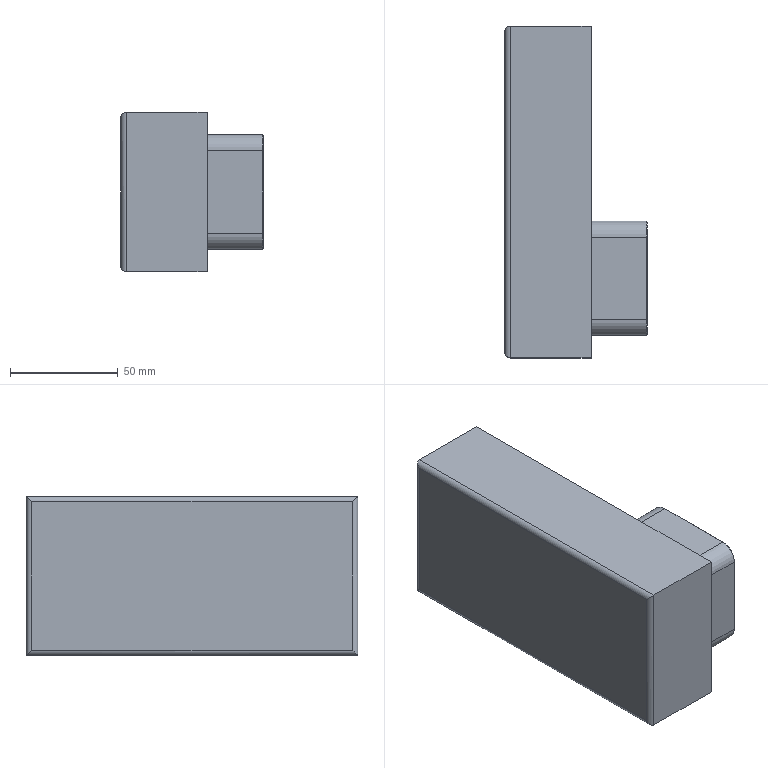Part | SolidWorks | features BaseBody 1 | 1 solid | 35 faces | box 66 x 153.7 x 73.7 mm | volume 524203 mm3 | plane 17 | cylinder 12 | cone 6 | commonest cylinder face diameters 5 x4 15 x4 8.8 x2 10 x2
STEP:
#1=CARTESIAN_POINT('',(-8.,26.2,-5.));
#2=VERTEX_POINT('',#1);
#3=CARTESIAN_POINT('',(-8.,26.2,5.));
#4=VERTEX_POINT('',#3);
#5=CARTESIAN_POINT('',(-8.,26.2,0.));
#6=DIRECTION('',(0.,1.,0.));
#7=DIRECTION('',(0.,0.,1.));
#8=AXIS2_PLACEMENT_3D('',#5,#6,#7);
#9=CIRCLE('',#8,5.);
#10=EDGE_CURVE('',#2,#4,#9,.T.);
#11=ORIENTED_EDGE('',*,*,#10,.F.);
#12=CARTESIAN_POINT('',(-8.,26.5,-5.3));
#13=VERTEX_POINT('',#12);
#14=CARTESIAN_POINT('',(-8.,26.5,-5.3));
#15=DIRECTION('',(0.,0.7071,-0.7071));
#16=VECTOR('',#15,1000.);
#17=LINE('',#14,#16);
#18=EDGE_CURVE('',#2,#13,#17,.T.);
#19=ORIENTED_EDGE('',*,*,#18,.T.);
#20=CARTESIAN_POINT('',(-8.,26.5,5.3));
#21=VERTEX_POINT('',#20);
#22=CARTESIAN_POINT('',(-8.,26.5,0.));
#23=DIRECTION('',(0.,-1.,0.));
#24=DIRECTION('',(0.,0.,1.));
#25=AXIS2_PLACEMENT_3D('',#22,#23,#24);
#26=CIRCLE('',#25,5.3);
#27=EDGE_CURVE('',#21,#13,#26,.T.);
#28=ORIENTED_EDGE('',*,*,#27,.F.);
#29=CARTESIAN_POINT('',(-8.,26.5,5.3));
#30=DIRECTION('',(0.,0.7071,0.7071));
#31=VECTOR('',#30,1000.);
#32=LINE('',#29,#31);
#33=EDGE_CURVE('',#4,#21,#32,.T.);
#34=ORIENTED_EDGE('',*,*,#33,.F.);
#35=EDGE_LOOP('',(#11,#19,#28,#34));
#36=FACE_OUTER_BOUND('',#35,.T.);
#37=CARTESIAN_POINT('',(-8.,26.5,0.));
#38=DIRECTION('',(0.,1.,0.));
#39=DIRECTION('',(0.,0.,1.));
#40=AXIS2_PLACEMENT_3D('',#37,#38,#39);
#41=CONICAL_SURFACE('',#40,5.3,0.7854);
#42=ADVANCED_FACE('',(#36),#41,.F.);
#43=CARTESIAN_POINT('',(-8.,23.5,-5.));
#44=VERTEX_POINT('',#43);
#45=CARTESIAN_POINT('',(-8.,23.5,5.));
#46=VERTEX_POINT('',#45);
#47=CARTESIAN_POINT('',(-8.,23.5,0.));
#48=DIRECTION('',(0.,1.,0.));
#49=DIRECTION('',(0.,0.,1.));
#50=AXIS2_PLACEMENT_3D('',#47,#48,#49);
#51=CIRCLE('',#50,5.);
#52=EDGE_CURVE('',#44,#46,#51,.T.);
#53=ORIENTED_EDGE('',*,*,#52,.F.);
#54=CARTESIAN_POINT('',(-8.,23.5,-5.));
#55=DIRECTION('',(0.,1.,0.));
#56=VECTOR('',#55,1000.);
#57=LINE('',#54,#56);
#58=EDGE_CURVE('',#44,#2,#57,.T.);
#59=ORIENTED_EDGE('',*,*,#58,.T.);
#60=ORIENTED_EDGE('',*,*,#10,.T.);
#61=CARTESIAN_POINT('',(-8.,23.5,5.));
#62=DIRECTION('',(0.,1.,0.));
#63=VECTOR('',#62,1000.);
#64=LINE('',#61,#63);
#65=EDGE_CURVE('',#46,#4,#64,.T.);
#66=ORIENTED_EDGE('',*,*,#65,.F.);
#67=EDGE_LOOP('',(#53,#59,#60,#66));
#68=FACE_OUTER_BOUND('',#67,.T.);
#69=CARTESIAN_POINT('',(-8.,23.5,0.));
#70=DIRECTION('',(0.,1.,0.));
#71=DIRECTION('',(0.,0.,1.));
#72=AXIS2_PLACEMENT_3D('',#69,#70,#71);
#73=CYLINDRICAL_SURFACE('',#72,5.);
#74=ADVANCED_FACE('',(#68),#73,.F.);
#75=CARTESIAN_POINT('',(-8.,23.5,-4.4));
#76=VERTEX_POINT('',#75);
#77=CARTESIAN_POINT('',(-8.,23.5,4.4));
#78=VERTEX_POINT('',#77);
#79=CARTESIAN_POINT('',(-8.,23.5,0.));
#80=DIRECTION('',(0.,-1.,0.));
#81=DIRECTION('',(0.,0.,1.));
#82=AXIS2_PLACEMENT_3D('',#79,#80,#81);
#83=CIRCLE('',#82,4.4);
#84=EDGE_CURVE('',#76,#78,#83,.T.);
#85=ORIENTED_EDGE('',*,*,#84,.F.);
#86=CARTESIAN_POINT('',(-8.,26.5,-4.4));
#87=VERTEX_POINT('',#86);
#88=CARTESIAN_POINT('',(-8.,23.5,-4.4));
#89=DIRECTION('',(0.,1.,0.));
#90=VECTOR('',#89,1000.);
#91=LINE('',#88,#90);
#92=EDGE_CURVE('',#76,#87,#91,.T.);
#93=ORIENTED_EDGE('',*,*,#92,.T.);
#94=CARTESIAN_POINT('',(-8.,26.5,4.4));
#95=VERTEX_POINT('',#94);
#96=CARTESIAN_POINT('',(-8.,26.5,0.));
#97=DIRECTION('',(0.,-1.,0.));
#98=DIRECTION('',(0.,0.,1.));
#99=AXIS2_PLACEMENT_3D('',#96,#97,#98);
#100=CIRCLE('',#99,4.4);
#101=EDGE_CURVE('',#87,#95,#100,.T.);
#102=ORIENTED_EDGE('',*,*,#101,.T.);
#103=CARTESIAN_POINT('',(-8.,23.5,4.4));
#104=DIRECTION('',(0.,1.,0.));
#105=VECTOR('',#104,1000.);
#106=LINE('',#103,#105);
#107=EDGE_CURVE('',#78,#95,#106,.T.);
#108=ORIENTED_EDGE('',*,*,#107,.F.);
#109=EDGE_LOOP('',(#85,#93,#102,#108));
#110=FACE_OUTER_BOUND('',#109,.T.);
#111=CARTESIAN_POINT('',(-8.,23.5,0.));
#112=DIRECTION('',(0.,1.,0.));
#113=DIRECTION('',(0.,0.,1.));
#114=AXIS2_PLACEMENT_3D('',#111,#112,#113);
#115=CYLINDRICAL_SURFACE('',#114,4.4);
#116=ADVANCED_FACE('',(#110),#115,.T.);
#117=CARTESIAN_POINT('',(-66.,114.35,34.35));
#118=VERTEX_POINT('',#117);
#119=CARTESIAN_POINT('',(-66.,-34.35,34.35));
#120=VERTEX_POINT('',#119);
#121=CARTESIAN_POINT('',(-66.,0.,34.35));
#122=DIRECTION('',(0.,-1.,0.));
#123=VECTOR('',#122,1000.);
#124=LINE('',#121,#123);
#125=EDGE_CURVE('',#118,#120,#124,.T.);
#126=ORIENTED_EDGE('',*,*,#125,.F.);
#127=CARTESIAN_POINT('',(-66.,114.35,-34.35));
#128=VERTEX_POINT('',#127);
#129=CARTESIAN_POINT('',(-66.,114.35,0.));
#130=DIRECTION('',(0.,0.,1.));
#131=VECTOR('',#130,1000.);
#132=LINE('',#129,#131);
#133=EDGE_CURVE('',#128,#118,#132,.T.);
#134=ORIENTED_EDGE('',*,*,#133,.F.);
#135=CARTESIAN_POINT('',(-66.,-34.35,-34.35));
#136=VERTEX_POINT('',#135);
#137=CARTESIAN_POINT('',(-66.,0.,-34.35));
#138=DIRECTION('',(0.,1.,0.));
#139=VECTOR('',#138,1000.);
#140=LINE('',#137,#139);
#141=EDGE_CURVE('',#136,#128,#140,.T.);
#142=ORIENTED_EDGE('',*,*,#141,.F.);
#143=CARTESIAN_POINT('',(-66.,-34.35,0.));
#144=DIRECTION('',(0.,0.,-1.));
#145=VECTOR('',#144,1000.);
#146=LINE('',#143,#145);
#147=EDGE_CURVE('',#120,#136,#146,.T.);
#148=ORIENTED_EDGE('',*,*,#147,.F.);
#149=EDGE_LOOP('',(#126,#134,#142,#148));
#150=FACE_OUTER_BOUND('',#149,.T.);
#151=CARTESIAN_POINT('',(-66.,0.,0.));
#152=DIRECTION('',(1.,0.,0.));
#153=DIRECTION('',(0.,0.,-1.));
#154=AXIS2_PLACEMENT_3D('',#151,#152,#153);
#155=PLANE('',#154);
#156=ADVANCED_FACE('',(#150),#155,.F.);
#157=CARTESIAN_POINT('',(-63.5,-36.85,36.85));
#158=VERTEX_POINT('',#157);
#159=CARTESIAN_POINT('',(-63.5,-36.85,36.85));
#160=CARTESIAN_POINT('',(-64.964,-36.85,36.85));
#161=CARTESIAN_POINT('',(-66.,-35.814,35.814));
#162=CARTESIAN_POINT('',(-66.,-34.35,34.35));
#163=(BOUNDED_CURVE()B_SPLINE_CURVE(3,(#159,#160,#161,#162),.UNSPECIFIED.,.F.,.F.)B_SPLINE_CURVE_WITH_KNOTS((4,4),(0.,1.571),.UNSPECIFIED.)CURVE()GEOMETRIC_REPRESENTATION_ITEM()RATIONAL_B_SPLINE_CURVE((1.,0.8047,0.8047,1.))REPRESENTATION_ITEM(''));
#164=EDGE_CURVE('',#158,#120,#163,.T.);
#165=ORIENTED_EDGE('',*,*,#164,.T.);
#166=ORIENTED_EDGE('',*,*,#147,.T.);
#167=CARTESIAN_POINT('',(-63.5,-36.85,-36.85));
#168=VERTEX_POINT('',#167);
#169=CARTESIAN_POINT('',(-66.,-34.35,-34.35));
#170=CARTESIAN_POINT('',(-66.,-35.814,-35.814));
#171=CARTESIAN_POINT('',(-64.964,-36.85,-36.85));
#172=CARTESIAN_POINT('',(-63.5,-36.85,-36.85));
#173=(BOUNDED_CURVE()B_SPLINE_CURVE(3,(#169,#170,#171,#172),.UNSPECIFIED.,.F.,.F.)B_SPLINE_CURVE_WITH_KNOTS((4,4),(1.571,3.142),.UNSPECIFIED.)CURVE()GEOMETRIC_REPRESENTATION_ITEM()RATIONAL_B_SPLINE_CURVE((1.,0.8047,0.8047,1.))REPRESENTATION_ITEM(''));
#174=EDGE_CURVE('',#136,#168,#173,.T.);
#175=ORIENTED_EDGE('',*,*,#174,.T.);
#176=CARTESIAN_POINT('',(-63.5,-36.85,36.85));
#177=DIRECTION('',(0.,0.,1.));
#178=VECTOR('',#177,1000.);
#179=LINE('',#176,#178);
#180=EDGE_CURVE('',#168,#158,#179,.T.);
#181=ORIENTED_EDGE('',*,*,#180,.T.);
#182=EDGE_LOOP('',(#165,#166,#175,#181));
#183=FACE_OUTER_BOUND('',#182,.T.);
#184=CARTESIAN_POINT('',(-63.5,-34.35,36.85));
#185=DIRECTION('',(0.,0.,1.));
#186=DIRECTION('',(0.,-1.,0.));
#187=AXIS2_PLACEMENT_3D('',#184,#185,#186);
#188=CYLINDRICAL_SURFACE('',#187,2.5);
#189=ADVANCED_FACE('',(#183),#188,.T.);
#190=ORIENTED_EDGE('',*,*,#164,.F.);
#191=CARTESIAN_POINT('',(-63.5,116.85,36.85));
#192=VERTEX_POINT('',#191);
#193=CARTESIAN_POINT('',(-63.5,116.85,36.85));
#194=DIRECTION('',(0.,1.,0.));
#195=VECTOR('',#194,1000.);
#196=LINE('',#193,#195);
#197=EDGE_CURVE('',#158,#192,#196,.T.);
#198=ORIENTED_EDGE('',*,*,#197,.T.);
#199=CARTESIAN_POINT('',(-63.5,116.85,36.85));
#200=CARTESIAN_POINT('',(-64.964,116.85,36.85));
#201=CARTESIAN_POINT('',(-66.,115.814,35.814));
#202=CARTESIAN_POINT('',(-66.,114.35,34.35));
#203=(BOUNDED_CURVE()B_SPLINE_CURVE(3,(#199,#200,#201,#202),.UNSPECIFIED.,.F.,.F.)B_SPLINE_CURVE_WITH_KNOTS((4,4),(0.,1.571),.UNSPECIFIED.)CURVE()GEOMETRIC_REPRESENTATION_ITEM()RATIONAL_B_SPLINE_CURVE((1.,0.8047,0.8047,1.))REPRESENTATION_ITEM(''));
#204=EDGE_CURVE('',#192,#118,#203,.T.);
#205=ORIENTED_EDGE('',*,*,#204,.T.);
#206=ORIENTED_EDGE('',*,*,#125,.T.);
#207=EDGE_LOOP('',(#190,#198,#205,#206));
#208=FACE_OUTER_BOUND('',#207,.T.);
#209=CARTESIAN_POINT('',(-63.5,116.85,34.35));
#210=DIRECTION('',(0.,1.,0.));
#211=DIRECTION('',(0.,0.,1.));
#212=AXIS2_PLACEMENT_3D('',#209,#210,#211);
#213=CYLINDRICAL_SURFACE('',#212,2.5);
#214=ADVANCED_FACE('',(#208),#213,.T.);
#215=ORIENTED_EDGE('',*,*,#204,.F.);
#216=CARTESIAN_POINT('',(-63.5,116.85,-36.85));
#217=VERTEX_POINT('',#216);
#218=CARTESIAN_POINT('',(-63.5,116.85,-36.85));
#219=DIRECTION('',(0.,0.,-1.));
#220=VECTOR('',#219,1000.);
#221=LINE('',#218,#220);
#222=EDGE_CURVE('',#192,#217,#221,.T.);
#223=ORIENTED_EDGE('',*,*,#222,.T.);
#224=CARTESIAN_POINT('',(-63.5,116.85,-36.85));
#225=CARTESIAN_POINT('',(-64.964,116.85,-36.85));
#226=CARTESIAN_POINT('',(-66.,115.814,-35.814));
#227=CARTESIAN_POINT('',(-66.,114.35,-34.35));
#228=(BOUNDED_CURVE()B_SPLINE_CURVE(3,(#224,#225,#226,#227),.UNSPECIFIED.,.F.,.F.)B_SPLINE_CURVE_WITH_KNOTS((4,4),(0.,1.571),.UNSPECIFIED.)CURVE()GEOMETRIC_REPRESENTATION_ITEM()RATIONAL_B_SPLINE_CURVE((1.,0.8047,0.8047,1.))REPRESENTATION_ITEM(''));
#229=EDGE_CURVE('',#217,#128,#228,.T.);
#230=ORIENTED_EDGE('',*,*,#229,.T.);
#231=ORIENTED_EDGE('',*,*,#133,.T.);
#232=EDGE_LOOP('',(#215,#223,#230,#231));
#233=FACE_OUTER_BOUND('',#232,.T.);
#234=CARTESIAN_POINT('',(-63.5,114.35,-36.85));
#235=DIRECTION('',(0.,0.,-1.));
#236=DIRECTION('',(-1.,0.,0.));
#237=AXIS2_PLACEMENT_3D('',#234,#235,#236);
#238=CYLINDRICAL_SURFACE('',#237,2.5);
#239=ADVANCED_FACE('',(#233),#238,.T.);
#240=ORIENTED_EDGE('',*,*,#229,.F.);
#241=CARTESIAN_POINT('',(-63.5,-36.85,-36.85));
#242=DIRECTION('',(0.,-1.,0.));
#243=VECTOR('',#242,1000.);
#244=LINE('',#241,#243);
#245=EDGE_CURVE('',#217,#168,#244,.T.);
#246=ORIENTED_EDGE('',*,*,#245,.T.);
#247=ORIENTED_EDGE('',*,*,#174,.F.);
#248=ORIENTED_EDGE('',*,*,#141,.T.);
#249=EDGE_LOOP('',(#240,#246,#247,#248));
#250=FACE_OUTER_BOUND('',#249,.T.);
#251=CARTESIAN_POINT('',(-63.5,-36.85,-34.35));
#252=DIRECTION('',(0.,-1.,0.));
#253=DIRECTION('',(0.,0.,-1.));
#254=AXIS2_PLACEMENT_3D('',#251,#252,#253);
#255=CYLINDRICAL_SURFACE('',#254,2.5);
#256=ADVANCED_FACE('',(#250),#255,.T.);
#257=CARTESIAN_POINT('',(-26.,-36.85,-36.85));
#258=VERTEX_POINT('',#257);
#259=CARTESIAN_POINT('',(-66.,-36.85,-36.85));
#260=DIRECTION('',(1.,0.,0.));
#261=VECTOR('',#260,1000.);
#262=LINE('',#259,#261);
#263=EDGE_CURVE('',#168,#258,#262,.T.);
#264=ORIENTED_EDGE('',*,*,#263,.T.);
#265=CARTESIAN_POINT('',(-26.,-36.85,36.85));
#266=VERTEX_POINT('',#265);
#267=CARTESIAN_POINT('',(-26.,-36.85,36.85));
#268=DIRECTION('',(0.,0.,1.));
#269=VECTOR('',#268,1000.);
#270=LINE('',#267,#269);
#271=EDGE_CURVE('',#258,#266,#270,.T.);
#272=ORIENTED_EDGE('',*,*,#271,.T.);
#273=CARTESIAN_POINT('',(-66.,-36.85,36.85));
#274=DIRECTION('',(-1.,0.,0.));
#275=VECTOR('',#274,1000.);
#276=LINE('',#273,#275);
#277=EDGE_CURVE('',#266,#158,#276,.T.);
#278=ORIENTED_EDGE('',*,*,#277,.T.);
#279=ORIENTED_EDGE('',*,*,#180,.F.);
#280=EDGE_LOOP('',(#264,#272,#278,#279));
#281=FACE_OUTER_BOUND('',#280,.T.);
#282=CARTESIAN_POINT('',(-66.,-36.85,36.85));
#283=DIRECTION('',(0.,-1.,0.));
#284=DIRECTION('',(0.,0.,-1.));
#285=AXIS2_PLACEMENT_3D('',#282,#283,#284);
#286=PLANE('',#285);
#287=ADVANCED_FACE('',(#281),#286,.T.);
#288=ORIENTED_EDGE('',*,*,#277,.F.);
#289=CARTESIAN_POINT('',(-26.,116.85,36.85));
#290=VERTEX_POINT('',#289);
#291=CARTESIAN_POINT('',(-26.,116.85,36.85));
#292=DIRECTION('',(0.,1.,0.));
#293=VECTOR('',#292,1000.);
#294=LINE('',#291,#293);
#295=EDGE_CURVE('',#266,#290,#294,.T.);
#296=ORIENTED_EDGE('',*,*,#295,.T.);
#297=CARTESIAN_POINT('',(-66.,116.85,36.85));
#298=DIRECTION('',(-1.,0.,0.));
#299=VECTOR('',#298,1000.);
#300=LINE('',#297,#299);
#301=EDGE_CURVE('',#290,#192,#300,.T.);
#302=ORIENTED_EDGE('',*,*,#301,.T.);
#303=ORIENTED_EDGE('',*,*,#197,.F.);
#304=EDGE_LOOP('',(#288,#296,#302,#303));
#305=FACE_OUTER_BOUND('',#304,.T.);
#306=CARTESIAN_POINT('',(-66.,116.85,36.85));
#307=DIRECTION('',(0.,0.,1.));
#308=DIRECTION('',(1.,0.,0.));
#309=AXIS2_PLACEMENT_3D('',#306,#307,#308);
#310=PLANE('',#309);
#311=ADVANCED_FACE('',(#305),#310,.T.);
#312=ORIENTED_EDGE('',*,*,#301,.F.);
#313=CARTESIAN_POINT('',(-26.,116.85,-36.85));
#314=VERTEX_POINT('',#313);
#315=CARTESIAN_POINT('',(-26.,116.85,-36.85));
#316=DIRECTION('',(0.,0.,-1.));
#317=VECTOR('',#316,1000.);
#318=LINE('',#315,#317);
#319=EDGE_CURVE('',#290,#314,#318,.T.);
#320=ORIENTED_EDGE('',*,*,#319,.T.);
#321=CARTESIAN_POINT('',(-66.,116.85,-36.85));
#322=DIRECTION('',(-1.,0.,0.));
#323=VECTOR('',#322,1000.);
#324=LINE('',#321,#323);
#325=EDGE_CURVE('',#314,#217,#324,.T.);
#326=ORIENTED_EDGE('',*,*,#325,.T.);
#327=ORIENTED_EDGE('',*,*,#222,.F.);
#328=EDGE_LOOP('',(#312,#320,#326,#327));
#329=FACE_OUTER_BOUND('',#328,.T.);
#330=CARTESIAN_POINT('',(-66.,116.85,-36.85));
#331=DIRECTION('',(0.,1.,0.));
#332=DIRECTION('',(0.,0.,1.));
#333=AXIS2_PLACEMENT_3D('',#330,#331,#332);
#334=PLANE('',#333);
#335=ADVANCED_FACE('',(#329),#334,.T.);
#336=ORIENTED_EDGE('',*,*,#325,.F.);
#337=CARTESIAN_POINT('',(-26.,-36.85,-36.85));
#338=DIRECTION('',(0.,-1.,0.));
#339=VECTOR('',#338,1000.);
#340=LINE('',#337,#339);
#341=EDGE_CURVE('',#314,#258,#340,.T.);
#342=ORIENTED_EDGE('',*,*,#341,.T.);
#343=ORIENTED_EDGE('',*,*,#263,.F.);
#344=ORIENTED_EDGE('',*,*,#245,.F.);
#345=EDGE_LOOP('',(#336,#342,#343,#344));
#346=FACE_OUTER_BOUND('',#345,.T.);
#347=CARTESIAN_POINT('',(-66.,-36.85,-36.85));
#348=DIRECTION('',(0.,0.,-1.));
#349=DIRECTION('',(-1.,0.,0.));
#350=AXIS2_PLACEMENT_3D('',#347,#348,#349);
#351=PLANE('',#350);
#352=ADVANCED_FACE('',(#346),#351,.T.);
#353=ORIENTED_EDGE('',*,*,#271,.F.);
#354=ORIENTED_EDGE('',*,*,#341,.F.);
#355=ORIENTED_EDGE('',*,*,#319,.F.);
#356=ORIENTED_EDGE('',*,*,#295,.F.);
#357=EDGE_LOOP('',(#353,#354,#355,#356));
#358=FACE_OUTER_BOUND('',#357,.T.);
#359=CARTESIAN_POINT('',(-26.,-26.5,-19.));
#360=VERTEX_POINT('',#359);
#361=CARTESIAN_POINT('',(-26.,-26.5,19.));
#362=VERTEX_POINT('',#361);
#363=CARTESIAN_POINT('',(-26.,-26.5,0.));
#364=DIRECTION('',(0.,0.,1.));
#365=VECTOR('',#364,1000.);
#366=LINE('',#363,#365);
#367=EDGE_CURVE('',#360,#362,#366,.T.);
#368=ORIENTED_EDGE('',*,*,#367,.T.);
#369=CARTESIAN_POINT('',(-26.,-19.,26.5));
#370=VERTEX_POINT('',#369);
#371=CARTESIAN_POINT('',(-26.,-19.,19.));
#372=DIRECTION('',(-1.,0.,0.));
#373=DIRECTION('',(0.,0.,-1.));
#374=AXIS2_PLACEMENT_3D('',#371,#372,#373);
#375=CIRCLE('',#374,7.5);
#376=EDGE_CURVE('',#362,#370,#375,.T.);
#377=ORIENTED_EDGE('',*,*,#376,.T.);
#378=CARTESIAN_POINT('',(-26.,19.,26.5));
#379=VERTEX_POINT('',#378);
#380=CARTESIAN_POINT('',(-26.,0.,26.5));
#381=DIRECTION('',(0.,1.,0.));
#382=VECTOR('',#381,1000.);
#383=LINE('',#380,#382);
#384=EDGE_CURVE('',#370,#379,#383,.T.);
#385=ORIENTED_EDGE('',*,*,#384,.T.);
#386=CARTESIAN_POINT('',(-26.,26.5,19.));
#387=VERTEX_POINT('',#386);
#388=CARTESIAN_POINT('',(-26.,19.,19.));
#389=DIRECTION('',(-1.,0.,0.));
#390=DIRECTION('',(0.,0.,-1.));
#391=AXIS2_PLACEMENT_3D('',#388,#389,#390);
#392=CIRCLE('',#391,7.5);
#393=EDGE_CURVE('',#379,#387,#392,.T.);
#394=ORIENTED_EDGE('',*,*,#393,.T.);
#395=CARTESIAN_POINT('',(-26.,26.5,-19.));
#396=VERTEX_POINT('',#395);
#397=CARTESIAN_POINT('',(-26.,26.5,0.));
#398=DIRECTION('',(0.,0.,-1.));
#399=VECTOR('',#398,1000.);
#400=LINE('',#397,#399);
#401=EDGE_CURVE('',#387,#396,#400,.T.);
#402=ORIENTED_EDGE('',*,*,#401,.T.);
#403=CARTESIAN_POINT('',(-26.,19.,-26.5));
#404=VERTEX_POINT('',#403);
#405=CARTESIAN_POINT('',(-26.,19.,-19.));
#406=DIRECTION('',(-1.,0.,0.));
#407=DIRECTION('',(0.,0.,-1.));
#408=AXIS2_PLACEMENT_3D('',#405,#406,#407);
#409=CIRCLE('',#408,7.5);
#410=EDGE_CURVE('',#396,#404,#409,.T.);
#411=ORIENTED_EDGE('',*,*,#410,.T.);
#412=CARTESIAN_POINT('',(-26.,-19.,-26.5));
#413=VERTEX_POINT('',#412);
#414=CARTESIAN_POINT('',(-26.,0.,-26.5));
#415=DIRECTION('',(0.,-1.,0.));
#416=VECTOR('',#415,1000.);
#417=LINE('',#414,#416);
#418=EDGE_CURVE('',#404,#413,#417,.T.);
#419=ORIENTED_EDGE('',*,*,#418,.T.);
#420=CARTESIAN_POINT('',(-26.,-19.,-19.));
#421=DIRECTION('',(-1.,0.,0.));
#422=DIRECTION('',(0.,0.,-1.));
#423=AXIS2_PLACEMENT_3D('',#420,#421,#422);
#424=CIRCLE('',#423,7.5);
#425=EDGE_CURVE('',#413,#360,#424,.T.);
#426=ORIENTED_EDGE('',*,*,#425,.T.);
#427=EDGE_LOOP('',(#368,#377,#385,#394,#402,#411,#419,#426));
#428=FACE_BOUND('',#427,.T.);
#429=CARTESIAN_POINT('',(-26.,0.,0.));
#430=DIRECTION('',(1.,0.,0.));
#431=DIRECTION('',(0.,0.,-1.));
#432=AXIS2_PLACEMENT_3D('',#429,#430,#431);
#433=PLANE('',#432);
#434=ADVANCED_FACE('',(#358,#428),#433,.T.);
#435=CARTESIAN_POINT('',(-0.5,-19.,26.5));
#436=VERTEX_POINT('',#435);
#437=CARTESIAN_POINT('',(-26.,-19.,26.5));
#438=DIRECTION('',(-1.,0.,0.));
#439=VECTOR('',#438,1000.);
#440=LINE('',#437,#439);
#441=EDGE_CURVE('',#436,#370,#440,.T.);
#442=ORIENTED_EDGE('',*,*,#441,.T.);
#443=ORIENTED_EDGE('',*,*,#376,.F.);
#444=CARTESIAN_POINT('',(-0.5,-26.5,19.));
#445=VERTEX_POINT('',#444);
#446=CARTESIAN_POINT('',(-26.,-26.5,19.));
#447=DIRECTION('',(1.,0.,0.));
#448=VECTOR('',#447,1000.);
#449=LINE('',#446,#448);
#450=EDGE_CURVE('',#362,#445,#449,.T.);
#451=ORIENTED_EDGE('',*,*,#450,.T.);
#452=CARTESIAN_POINT('',(-0.5,-19.,19.));
#453=DIRECTION('',(-1.,0.,0.));
#454=DIRECTION('',(0.,0.,-1.));
#455=AXIS2_PLACEMENT_3D('',#452,#453,#454);
#456=CIRCLE('',#455,7.5);
#457=EDGE_CURVE('',#445,#436,#456,.T.);
#458=ORIENTED_EDGE('',*,*,#457,.T.);
#459=EDGE_LOOP('',(#442,#443,#451,#458));
#460=FACE_OUTER_BOUND('',#459,.T.);
#461=CARTESIAN_POINT('',(-26.,-19.,19.));
#462=DIRECTION('',(1.,0.,0.));
#463=DIRECTION('',(0.,0.,-1.));
#464=AXIS2_PLACEMENT_3D('',#461,#462,#463);
#465=CYLINDRICAL_SURFACE('',#464,7.5);
#466=ADVANCED_FACE('',(#460),#465,.T.);
#467=ORIENTED_EDGE('',*,*,#450,.F.);
#468=ORIENTED_EDGE('',*,*,#367,.F.);
#469=CARTESIAN_POINT('',(-0.5,-26.5,-19.));
#470=VERTEX_POINT('',#469);
#471=CARTESIAN_POINT('',(-26.,-26.5,-19.));
#472=DIRECTION('',(1.,0.,0.));
#473=VECTOR('',#472,1000.);
#474=LINE('',#471,#473);
#475=EDGE_CURVE('',#360,#470,#474,.T.);
#476=ORIENTED_EDGE('',*,*,#475,.T.);
#477=CARTESIAN_POINT('',(-0.5,-26.5,19.));
#478=DIRECTION('',(0.,0.,1.));
#479=VECTOR('',#478,1000.);
#480=LINE('',#477,#479);
#481=EDGE_CURVE('',#470,#445,#480,.T.);
#482=ORIENTED_EDGE('',*,*,#481,.T.);
#483=EDGE_LOOP('',(#467,#468,#476,#482));
#484=FACE_OUTER_BOUND('',#483,.T.);
#485=CARTESIAN_POINT('',(-26.,-26.5,19.));
#486=DIRECTION('',(0.,-1.,0.));
#487=DIRECTION('',(0.,0.,-1.));
#488=AXIS2_PLACEMENT_3D('',#485,#486,#487);
#489=PLANE('',#488);
#490=ADVANCED_FACE('',(#484),#489,.T.);
#491=ORIENTED_EDGE('',*,*,#475,.F.);
#492=ORIENTED_EDGE('',*,*,#425,.F.);
#493=CARTESIAN_POINT('',(-0.5,-19.,-26.5));
#494=VERTEX_POINT('',#493);
#495=CARTESIAN_POINT('',(-26.,-19.,-26.5));
#496=DIRECTION('',(1.,0.,0.));
#497=VECTOR('',#496,1000.);
#498=LINE('',#495,#497);
#499=EDGE_CURVE('',#413,#494,#498,.T.);
#500=ORIENTED_EDGE('',*,*,#499,.T.);
#501=CARTESIAN_POINT('',(-0.5,-19.,-19.));
#502=DIRECTION('',(-1.,0.,0.));
#503=DIRECTION('',(0.,0.,-1.));
#504=AXIS2_PLACEMENT_3D('',#501,#502,#503);
#505=CIRCLE('',#504,7.5);
#506=EDGE_CURVE('',#494,#470,#505,.T.);
#507=ORIENTED_EDGE('',*,*,#506,.T.);
#508=EDGE_LOOP('',(#491,#492,#500,#507));
#509=FACE_OUTER_BOUND('',#508,.T.);
#510=CARTESIAN_POINT('',(-26.,-19.,-19.));
#511=DIRECTION('',(1.,0.,0.));
#512=DIRECTION('',(0.,0.,-1.));
#513=AXIS2_PLACEMENT_3D('',#510,#511,#512);
#514=CYLINDRICAL_SURFACE('',#513,7.5);
#515=ADVANCED_FACE('',(#509),#514,.T.);
#516=ORIENTED_EDGE('',*,*,#499,.F.);
#517=ORIENTED_EDGE('',*,*,#418,.F.);
#518=CARTESIAN_POINT('',(-0.5,19.,-26.5));
#519=VERTEX_POINT('',#518);
#520=CARTESIAN_POINT('',(-26.,19.,-26.5));
#521=DIRECTION('',(1.,0.,0.));
#522=VECTOR('',#521,1000.);
#523=LINE('',#520,#522);
#524=EDGE_CURVE('',#404,#519,#523,.T.);
#525=ORIENTED_EDGE('',*,*,#524,.T.);
#526=CARTESIAN_POINT('',(-0.5,-19.,-26.5));
#527=DIRECTION('',(0.,-1.,0.));
#528=VECTOR('',#527,1000.);
#529=LINE('',#526,#528);
#530=EDGE_CURVE('',#519,#494,#529,.T.);
#531=ORIENTED_EDGE('',*,*,#530,.T.);
#532=EDGE_LOOP('',(#516,#517,#525,#531));
#533=FACE_OUTER_BOUND('',#532,.T.);
#534=CARTESIAN_POINT('',(-26.,-19.,-26.5));
#535=DIRECTION('',(0.,0.,-1.));
#536=DIRECTION('',(-1.,0.,0.));
#537=AXIS2_PLACEMENT_3D('',#534,#535,#536);
#538=PLANE('',#537);
#539=ADVANCED_FACE('',(#533),#538,.T.);
#540=ORIENTED_EDGE('',*,*,#524,.F.);
#541=ORIENTED_EDGE('',*,*,#410,.F.);
#542=CARTESIAN_POINT('',(-0.5,26.5,-19.));
#543=VERTEX_POINT('',#542);
#544=CARTESIAN_POINT('',(-26.,26.5,-19.));
#545=DIRECTION('',(1.,0.,0.));
#546=VECTOR('',#545,1000.);
#547=LINE('',#544,#546);
#548=EDGE_CURVE('',#396,#543,#547,.T.);
#549=ORIENTED_EDGE('',*,*,#548,.T.);
#550=CARTESIAN_POINT('',(-0.5,19.,-19.));
#551=DIRECTION('',(-1.,0.,0.));
#552=DIRECTION('',(0.,0.,-1.));
#553=AXIS2_PLACEMENT_3D('',#550,#551,#552);
#554=CIRCLE('',#553,7.5);
#555=EDGE_CURVE('',#543,#519,#554,.T.);
#556=ORIENTED_EDGE('',*,*,#555,.T.);
#557=EDGE_LOOP('',(#540,#541,#549,#556));
#558=FACE_OUTER_BOUND('',#557,.T.);
#559=CARTESIAN_POINT('',(-26.,19.,-19.));
#560=DIRECTION('',(1.,0.,0.));
#561=DIRECTION('',(0.,0.,-1.));
#562=AXIS2_PLACEMENT_3D('',#559,#560,#561);
#563=CYLINDRICAL_SURFACE('',#562,7.5);
#564=ADVANCED_FACE('',(#558),#563,.T.);
#565=ORIENTED_EDGE('',*,*,#548,.F.);
#566=ORIENTED_EDGE('',*,*,#401,.F.);
#567=CARTESIAN_POINT('',(-0.5,26.5,19.));
#568=VERTEX_POINT('',#567);
#569=CARTESIAN_POINT('',(-26.,26.5,19.));
#570=DIRECTION('',(1.,0.,0.));
#571=VECTOR('',#570,1000.);
#572=LINE('',#569,#571);
#573=EDGE_CURVE('',#387,#568,#572,.T.);
#574=ORIENTED_EDGE('',*,*,#573,.T.);
#575=CARTESIAN_POINT('',(-0.5,26.5,-19.));
#576=DIRECTION('',(0.,0.,-1.));
#577=VECTOR('',#576,1000.);
#578=LINE('',#575,#577);
#579=EDGE_CURVE('',#568,#543,#578,.T.);
#580=ORIENTED_EDGE('',*,*,#579,.T.);
#581=EDGE_LOOP('',(#565,#566,#574,#580));
#582=FACE_OUTER_BOUND('',#581,.T.);
#583=ORIENTED_EDGE('',*,*,#27,.T.);
#584=CARTESIAN_POINT('',(-8.,26.5,0.));
#585=DIRECTION('',(0.,-1.,0.));
#586=DIRECTION('',(0.,0.,1.));
#587=AXIS2_PLACEMENT_3D('',#584,#585,#586);
#588=CIRCLE('',#587,5.3);
#589=EDGE_CURVE('',#13,#21,#588,.T.);
#590=ORIENTED_EDGE('',*,*,#589,.T.);
#591=EDGE_LOOP('',(#583,#590));
#592=FACE_BOUND('',#591,.T.);
#593=CARTESIAN_POINT('',(-26.,26.5,-19.));
#594=DIRECTION('',(0.,1.,0.));
#595=DIRECTION('',(0.,0.,1.));
#596=AXIS2_PLACEMENT_3D('',#593,#594,#595);
#597=PLANE('',#596);
#598=ADVANCED_FACE('',(#582,#592),#597,.T.);
#599=ORIENTED_EDGE('',*,*,#573,.F.);
#600=ORIENTED_EDGE('',*,*,#393,.F.);
#601=CARTESIAN_POINT('',(-0.5,19.,26.5));
#602=VERTEX_POINT('',#601);
#603=CARTESIAN_POINT('',(-26.,19.,26.5));
#604=DIRECTION('',(1.,0.,0.));
#605=VECTOR('',#604,1000.);
#606=LINE('',#603,#605);
#607=EDGE_CURVE('',#379,#602,#606,.T.);
#608=ORIENTED_EDGE('',*,*,#607,.T.);
#609=CARTESIAN_POINT('',(-0.5,19.,19.));
#610=DIRECTION('',(-1.,0.,0.));
#611=DIRECTION('',(0.,0.,-1.));
#612=AXIS2_PLACEMENT_3D('',#609,#610,#611);
#613=CIRCLE('',#612,7.5);
#614=EDGE_CURVE('',#602,#568,#613,.T.);
#615=ORIENTED_EDGE('',*,*,#614,.T.);
#616=EDGE_LOOP('',(#599,#600,#608,#615));
#617=FACE_OUTER_BOUND('',#616,.T.);
#618=CARTESIAN_POINT('',(-26.,19.,19.));
#619=DIRECTION('',(1.,0.,0.));
#620=DIRECTION('',(0.,0.,-1.));
#621=AXIS2_PLACEMENT_3D('',#618,#619,#620);
#622=CYLINDRICAL_SURFACE('',#621,7.5);
#623=ADVANCED_FACE('',(#617),#622,.T.);
#624=ORIENTED_EDGE('',*,*,#607,.F.);
#625=ORIENTED_EDGE('',*,*,#384,.F.);
#626=ORIENTED_EDGE('',*,*,#441,.F.);
#627=CARTESIAN_POINT('',(-0.5,19.,26.5));
#628=DIRECTION('',(0.,1.,0.));
#629=VECTOR('',#628,1000.);
#630=LINE('',#627,#629);
#631=EDGE_CURVE('',#436,#602,#630,.T.);
#632=ORIENTED_EDGE('',*,*,#631,.T.);
#633=EDGE_LOOP('',(#624,#625,#626,#632));
#634=FACE_OUTER_BOUND('',#633,.T.);
#635=CARTESIAN_POINT('',(-26.,19.,26.5));
#636=DIRECTION('',(0.,0.,1.));
#637=DIRECTION('',(1.,0.,0.));
#638=AXIS2_PLACEMENT_3D('',#635,#636,#637);
#639=PLANE('',#638);
#640=ADVANCED_FACE('',(#634),#639,.T.);
#641=CARTESIAN_POINT('',(0.,-19.,26.));
#642=VERTEX_POINT('',#641);
#643=CARTESIAN_POINT('',(-498974.,-19.,499000.));
#644=DIRECTION('',(-0.7071,0.,0.7071));
#645=VECTOR('',#644,1000.);
#646=LINE('',#643,#645);
#647=EDGE_CURVE('',#642,#436,#646,.T.);
#648=ORIENTED_EDGE('',*,*,#647,.T.);
#649=ORIENTED_EDGE('',*,*,#457,.F.);
#650=CARTESIAN_POINT('',(0.,-26.,19.));
#651=VERTEX_POINT('',#650);
#652=CARTESIAN_POINT('',(-498974.,-499000.,19.));
#653=DIRECTION('',(0.7071,0.7071,0.));
#654=VECTOR('',#653,1000.);
#655=LINE('',#652,#654);
#656=EDGE_CURVE('',#445,#651,#655,.T.);
#657=ORIENTED_EDGE('',*,*,#656,.T.);
#658=CARTESIAN_POINT('',(0.,-19.,19.));
#659=DIRECTION('',(-1.,0.,0.));
#660=DIRECTION('',(0.,0.,1.));
#661=AXIS2_PLACEMENT_3D('',#658,#659,#660);
#662=CIRCLE('',#661,7.);
#663=EDGE_CURVE('',#651,#642,#662,.T.);
#664=ORIENTED_EDGE('',*,*,#663,.T.);
#665=EDGE_LOOP('',(#648,#649,#657,#664));
#666=FACE_OUTER_BOUND('',#665,.T.);
#667=CARTESIAN_POINT('',(-0.5,-19.,19.));
#668=DIRECTION('',(-1.,0.,0.));
#669=DIRECTION('',(0.,0.,1.));
#670=AXIS2_PLACEMENT_3D('',#667,#668,#669);
#671=CONICAL_SURFACE('',#670,7.5,0.7854);
#672=ADVANCED_FACE('',(#666),#671,.T.);
#673=CARTESIAN_POINT('',(0.,-26.,-19.));
#674=VERTEX_POINT('',#673);
#675=CARTESIAN_POINT('',(0.,-26.,19.));
#676=DIRECTION('',(0.,0.,-1.));
#677=VECTOR('',#676,1000.);
#678=LINE('',#675,#677);
#679=EDGE_CURVE('',#651,#674,#678,.T.);
#680=ORIENTED_EDGE('',*,*,#679,.F.);
#681=ORIENTED_EDGE('',*,*,#656,.F.);
#682=ORIENTED_EDGE('',*,*,#481,.F.);
#683=CARTESIAN_POINT('',(0.,-26.,-19.));
#684=DIRECTION('',(-0.7071,-0.7071,0.));
#685=VECTOR('',#684,1000.);
#686=LINE('',#683,#685);
#687=EDGE_CURVE('',#674,#470,#686,.T.);
#688=ORIENTED_EDGE('',*,*,#687,.F.);
#689=EDGE_LOOP('',(#680,#681,#682,#688));
#690=FACE_OUTER_BOUND('',#689,.T.);
#691=CARTESIAN_POINT('',(0.,-26.,19.));
#692=DIRECTION('',(-0.7071,0.7071,0.));
#693=DIRECTION('',(-0.7071,-0.7071,0.));
#694=AXIS2_PLACEMENT_3D('',#691,#692,#693);
#695=PLANE('',#694);
#696=ADVANCED_FACE('',(#690),#695,.F.);
#697=CARTESIAN_POINT('',(0.,-19.,-26.));
#698=VERTEX_POINT('',#697);
#699=CARTESIAN_POINT('',(-499000.,-19.,-499026.));
#700=DIRECTION('',(0.7071,0.,0.7071));
#701=VECTOR('',#700,1000.);
#702=LINE('',#699,#701);
#703=EDGE_CURVE('',#494,#698,#702,.T.);
#704=ORIENTED_EDGE('',*,*,#703,.T.);
#705=CARTESIAN_POINT('',(0.,-19.,-19.));
#706=DIRECTION('',(-1.,0.,0.));
#707=DIRECTION('',(0.,0.,1.));
#708=AXIS2_PLACEMENT_3D('',#705,#706,#707);
#709=CIRCLE('',#708,7.);
#710=EDGE_CURVE('',#698,#674,#709,.T.);
#711=ORIENTED_EDGE('',*,*,#710,.T.);
#712=ORIENTED_EDGE('',*,*,#687,.T.);
#713=ORIENTED_EDGE('',*,*,#506,.F.);
#714=EDGE_LOOP('',(#704,#711,#712,#713));
#715=FACE_OUTER_BOUND('',#714,.T.);
#716=CARTESIAN_POINT('',(-0.5,-19.,-19.));
#717=DIRECTION('',(-1.,0.,0.));
#718=DIRECTION('',(0.,0.,1.));
#719=AXIS2_PLACEMENT_3D('',#716,#717,#718);
#720=CONICAL_SURFACE('',#719,7.5,0.7854);
#721=ADVANCED_FACE('',(#715),#720,.T.);
#722=ORIENTED_EDGE('',*,*,#530,.F.);
#723=CARTESIAN_POINT('',(0.,19.,-26.));
#724=VERTEX_POINT('',#723);
#725=CARTESIAN_POINT('',(0.,19.,-26.));
#726=DIRECTION('',(-0.7071,0.,-0.7071));
#727=VECTOR('',#726,1000.);
#728=LINE('',#725,#727);
#729=EDGE_CURVE('',#724,#519,#728,.T.);
#730=ORIENTED_EDGE('',*,*,#729,.F.);
#731=CARTESIAN_POINT('',(0.,-19.,-26.));
#732=DIRECTION('',(0.,1.,0.));
#733=VECTOR('',#732,1000.);
#734=LINE('',#731,#733);
#735=EDGE_CURVE('',#698,#724,#734,.T.);
#736=ORIENTED_EDGE('',*,*,#735,.F.);
#737=ORIENTED_EDGE('',*,*,#703,.F.);
#738=EDGE_LOOP('',(#722,#730,#736,#737));
#739=FACE_OUTER_BOUND('',#738,.T.);
#740=CARTESIAN_POINT('',(0.,-19.,-26.));
#741=DIRECTION('',(-0.7071,0.,0.7071));
#742=DIRECTION('',(0.7071,0.,0.7071));
#743=AXIS2_PLACEMENT_3D('',#740,#741,#742);
#744=PLANE('',#743);
#745=ADVANCED_FACE('',(#739),#744,.F.);
#746=CARTESIAN_POINT('',(0.,26.,-19.));
#747=VERTEX_POINT('',#746);
#748=CARTESIAN_POINT('',(-499000.,499026.,-19.));
#749=DIRECTION('',(0.7071,-0.7071,0.));
#750=VECTOR('',#749,1000.);
#751=LINE('',#748,#750);
#752=EDGE_CURVE('',#543,#747,#751,.T.);
#753=ORIENTED_EDGE('',*,*,#752,.T.);
#754=CARTESIAN_POINT('',(0.,19.,-19.));
#755=DIRECTION('',(-1.,0.,0.));
#756=DIRECTION('',(0.,0.,1.));
#757=AXIS2_PLACEMENT_3D('',#754,#755,#756);
#758=CIRCLE('',#757,7.);
#759=EDGE_CURVE('',#747,#724,#758,.T.);
#760=ORIENTED_EDGE('',*,*,#759,.T.);
#761=ORIENTED_EDGE('',*,*,#729,.T.);
#762=ORIENTED_EDGE('',*,*,#555,.F.);
#763=EDGE_LOOP('',(#753,#760,#761,#762));
#764=FACE_OUTER_BOUND('',#763,.T.);
#765=CARTESIAN_POINT('',(-0.5,19.,-19.));
#766=DIRECTION('',(-1.,0.,0.));
#767=DIRECTION('',(0.,0.,1.));
#768=AXIS2_PLACEMENT_3D('',#765,#766,#767);
#769=CONICAL_SURFACE('',#768,7.5,0.7854);
#770=ADVANCED_FACE('',(#764),#769,.T.);
#771=ORIENTED_EDGE('',*,*,#579,.F.);
#772=CARTESIAN_POINT('',(0.,26.,19.));
#773=VERTEX_POINT('',#772);
#774=CARTESIAN_POINT('',(0.,26.,19.));
#775=DIRECTION('',(-0.7071,0.7071,0.));
#776=VECTOR('',#775,1000.);
#777=LINE('',#774,#776);
#778=EDGE_CURVE('',#773,#568,#777,.T.);
#779=ORIENTED_EDGE('',*,*,#778,.F.);
#780=CARTESIAN_POINT('',(0.,26.,19.));
#781=DIRECTION('',(0.,0.,1.));
#782=VECTOR('',#781,1000.);
#783=LINE('',#780,#782);
#784=EDGE_CURVE('',#747,#773,#783,.T.);
#785=ORIENTED_EDGE('',*,*,#784,.F.);
#786=ORIENTED_EDGE('',*,*,#752,.F.);
#787=EDGE_LOOP('',(#771,#779,#785,#786));
#788=FACE_OUTER_BOUND('',#787,.T.);
#789=CARTESIAN_POINT('',(0.,26.,19.));
#790=DIRECTION('',(-0.7071,-0.7071,0.));
#791=DIRECTION('',(0.7071,-0.7071,0.));
#792=AXIS2_PLACEMENT_3D('',#789,#790,#791);
#793=PLANE('',#792);
#794=ADVANCED_FACE('',(#788),#793,.F.);
#795=ORIENTED_EDGE('',*,*,#18,.F.);
#796=CARTESIAN_POINT('',(-8.,26.2,0.));
#797=DIRECTION('',(0.,1.,0.));
#798=DIRECTION('',(0.,0.,1.));
#799=AXIS2_PLACEMENT_3D('',#796,#797,#798);
#800=CIRCLE('',#799,5.);
#801=EDGE_CURVE('',#4,#2,#800,.T.);
#802=ORIENTED_EDGE('',*,*,#801,.F.);
#803=ORIENTED_EDGE('',*,*,#33,.T.);
#804=ORIENTED_EDGE('',*,*,#589,.F.);
#805=EDGE_LOOP('',(#795,#802,#803,#804));
#806=FACE_OUTER_BOUND('',#805,.T.);
#807=CARTESIAN_POINT('',(-8.,26.5,0.));
#808=DIRECTION('',(0.,1.,0.));
#809=DIRECTION('',(0.,0.,1.));
#810=AXIS2_PLACEMENT_3D('',#807,#808,#809);
#811=CONICAL_SURFACE('',#810,5.3,0.7854);
#812=ADVANCED_FACE('',(#806),#811,.F.);
#813=CARTESIAN_POINT('',(0.,19.,26.));
#814=VERTEX_POINT('',#813);
#815=CARTESIAN_POINT('',(-498974.,19.,499000.));
#816=DIRECTION('',(0.7071,0.,-0.7071));
#817=VECTOR('',#816,1000.);
#818=LINE('',#815,#817);
#819=EDGE_CURVE('',#602,#814,#818,.T.);
#820=ORIENTED_EDGE('',*,*,#819,.T.);
#821=CARTESIAN_POINT('',(0.,19.,19.));
#822=DIRECTION('',(-1.,0.,0.));
#823=DIRECTION('',(0.,0.,1.));
#824=AXIS2_PLACEMENT_3D('',#821,#822,#823);
#825=CIRCLE('',#824,7.);
#826=EDGE_CURVE('',#814,#773,#825,.T.);
#827=ORIENTED_EDGE('',*,*,#826,.T.);
#828=ORIENTED_EDGE('',*,*,#778,.T.);
#829=ORIENTED_EDGE('',*,*,#614,.F.);
#830=EDGE_LOOP('',(#820,#827,#828,#829));
#831=FACE_OUTER_BOUND('',#830,.T.);
#832=CARTESIAN_POINT('',(-0.5,19.,19.));
#833=DIRECTION('',(-1.,0.,0.));
#834=DIRECTION('',(0.,0.,1.));
#835=AXIS2_PLACEMENT_3D('',#832,#833,#834);
#836=CONICAL_SURFACE('',#835,7.5,0.7854);
#837=ADVANCED_FACE('',(#831),#836,.T.);
#838=CARTESIAN_POINT('',(0.,-19.,26.));
#839=DIRECTION('',(0.,-1.,0.));
#840=VECTOR('',#839,1000.);
#841=LINE('',#838,#840);
#842=EDGE_CURVE('',#814,#642,#841,.T.);
#843=ORIENTED_EDGE('',*,*,#842,.F.);
#844=ORIENTED_EDGE('',*,*,#819,.F.);
#845=ORIENTED_EDGE('',*,*,#631,.F.);
#846=ORIENTED_EDGE('',*,*,#647,.F.);
#847=EDGE_LOOP('',(#843,#844,#845,#846));
#848=FACE_OUTER_BOUND('',#847,.T.);
#849=CARTESIAN_POINT('',(0.,-19.,26.));
#850=DIRECTION('',(-0.7071,0.,-0.7071));
#851=DIRECTION('',(-0.7071,0.,0.7071));
#852=AXIS2_PLACEMENT_3D('',#849,#850,#851);
#853=PLANE('',#852);
#854=ADVANCED_FACE('',(#848),#853,.F.);
#855=ORIENTED_EDGE('',*,*,#735,.T.);
#856=ORIENTED_EDGE('',*,*,#759,.F.);
#857=ORIENTED_EDGE('',*,*,#784,.T.);
#858=ORIENTED_EDGE('',*,*,#826,.F.);
#859=ORIENTED_EDGE('',*,*,#842,.T.);
#860=ORIENTED_EDGE('',*,*,#663,.F.);
#861=ORIENTED_EDGE('',*,*,#679,.T.);
#862=ORIENTED_EDGE('',*,*,#710,.F.);
#863=EDGE_LOOP('',(#855,#856,#857,#858,#859,#860,#861,#862));
#864=FACE_OUTER_BOUND('',#863,.T.);
#865=CARTESIAN_POINT('',(0.,-19.,19.));
#866=DIRECTION('',(1.,0.,0.));
#867=DIRECTION('',(0.,0.,-1.));
#868=AXIS2_PLACEMENT_3D('',#865,#866,#867);
#869=PLANE('',#868);
#870=ADVANCED_FACE('',(#864),#869,.T.);
#871=ORIENTED_EDGE('',*,*,#58,.F.);
#872=CARTESIAN_POINT('',(-8.,23.5,0.));
#873=DIRECTION('',(0.,1.,0.));
#874=DIRECTION('',(0.,0.,1.));
#875=AXIS2_PLACEMENT_3D('',#872,#873,#874);
#876=CIRCLE('',#875,5.);
#877=EDGE_CURVE('',#46,#44,#876,.T.);
#878=ORIENTED_EDGE('',*,*,#877,.F.);
#879=ORIENTED_EDGE('',*,*,#65,.T.);
#880=ORIENTED_EDGE('',*,*,#801,.T.);
#881=EDGE_LOOP('',(#871,#878,#879,#880));
#882=FACE_OUTER_BOUND('',#881,.T.);
#883=CARTESIAN_POINT('',(-8.,23.5,0.));
#884=DIRECTION('',(0.,1.,0.));
#885=DIRECTION('',(0.,0.,1.));
#886=AXIS2_PLACEMENT_3D('',#883,#884,#885);
#887=CYLINDRICAL_SURFACE('',#886,5.);
#888=ADVANCED_FACE('',(#882),#887,.F.);
#889=ORIENTED_EDGE('',*,*,#877,.T.);
#890=ORIENTED_EDGE('',*,*,#52,.T.);
#891=EDGE_LOOP('',(#889,#890));
#892=FACE_OUTER_BOUND('',#891,.T.);
#893=CARTESIAN_POINT('',(-8.,23.5,0.));
#894=DIRECTION('',(0.,-1.,0.));
#895=DIRECTION('',(0.,0.,1.));
#896=AXIS2_PLACEMENT_3D('',#893,#894,#895);
#897=CIRCLE('',#896,4.4);
#898=EDGE_CURVE('',#78,#76,#897,.T.);
#899=ORIENTED_EDGE('',*,*,#898,.T.);
#900=ORIENTED_EDGE('',*,*,#84,.T.);
#901=EDGE_LOOP('',(#899,#900));
#902=FACE_BOUND('',#901,.T.);
#903=CARTESIAN_POINT('',(-8.,23.5,0.));
#904=DIRECTION('',(0.,1.,0.));
#905=DIRECTION('',(0.,0.,1.));
#906=AXIS2_PLACEMENT_3D('',#903,#904,#905);
#907=PLANE('',#906);
#908=ADVANCED_FACE('',(#892,#902),#907,.T.);
#909=ORIENTED_EDGE('',*,*,#92,.F.);
#910=ORIENTED_EDGE('',*,*,#898,.F.);
#911=ORIENTED_EDGE('',*,*,#107,.T.);
#912=CARTESIAN_POINT('',(-8.,26.5,0.));
#913=DIRECTION('',(0.,-1.,0.));
#914=DIRECTION('',(0.,0.,1.));
#915=AXIS2_PLACEMENT_3D('',#912,#913,#914);
#916=CIRCLE('',#915,4.4);
#917=EDGE_CURVE('',#95,#87,#916,.T.);
#918=ORIENTED_EDGE('',*,*,#917,.T.);
#919=EDGE_LOOP('',(#909,#910,#911,#918));
#920=FACE_OUTER_BOUND('',#919,.T.);
#921=CARTESIAN_POINT('',(-8.,23.5,0.));
#922=DIRECTION('',(0.,1.,0.));
#923=DIRECTION('',(0.,0.,1.));
#924=AXIS2_PLACEMENT_3D('',#921,#922,#923);
#925=CYLINDRICAL_SURFACE('',#924,4.4);
#926=ADVANCED_FACE('',(#920),#925,.T.);
#927=ORIENTED_EDGE('',*,*,#917,.F.);
#928=ORIENTED_EDGE('',*,*,#101,.F.);
#929=EDGE_LOOP('',(#927,#928));
#930=FACE_OUTER_BOUND('',#929,.T.);
#931=CARTESIAN_POINT('',(-8.,26.5,0.));
#932=DIRECTION('',(0.,1.,0.));
#933=DIRECTION('',(0.,0.,1.));
#934=AXIS2_PLACEMENT_3D('',#931,#932,#933);
#935=PLANE('',#934);
#936=ADVANCED_FACE('',(#930),#935,.T.);
#937=CLOSED_SHELL('',(#42,#74,#116,#156,#189,#214,#239,#256,#287,#311,#335,#352,#434,#466,#490,#515,#539,#564,#598,#623,#640,#672,#696,#721,#745,#770,#794,#812,#837,#854,#870,#888,#908,#926,#936));
#938=MANIFOLD_SOLID_BREP('',#937);
#939=CARTESIAN_POINT('',(0.,0.,0.));
#940=DIRECTION('',(0.,0.,1.));
#941=DIRECTION('',(1.,0.,0.));
#942=AXIS2_PLACEMENT_3D('',#939,#940,#941);
#943=(LENGTH_UNIT()NAMED_UNIT(*)SI_UNIT(.MILLI.,.METRE.));
#944=UNCERTAINTY_MEASURE_WITH_UNIT(LENGTH_MEASURE(0.00001),#943,'','');
#945=(NAMED_UNIT(*)PLANE_ANGLE_UNIT()SI_UNIT($,.RADIAN.));
#946=(NAMED_UNIT(*)SI_UNIT($,.STERADIAN.)SOLID_ANGLE_UNIT());
#947=(GEOMETRIC_REPRESENTATION_CONTEXT(3)GLOBAL_UNCERTAINTY_ASSIGNED_CONTEXT((#944))GLOBAL_UNIT_ASSIGNED_CONTEXT((#943,#945,#946))REPRESENTATION_CONTEXT('',''));
#948=ADVANCED_BREP_SHAPE_REPRESENTATION('',(#938,#942),#947);